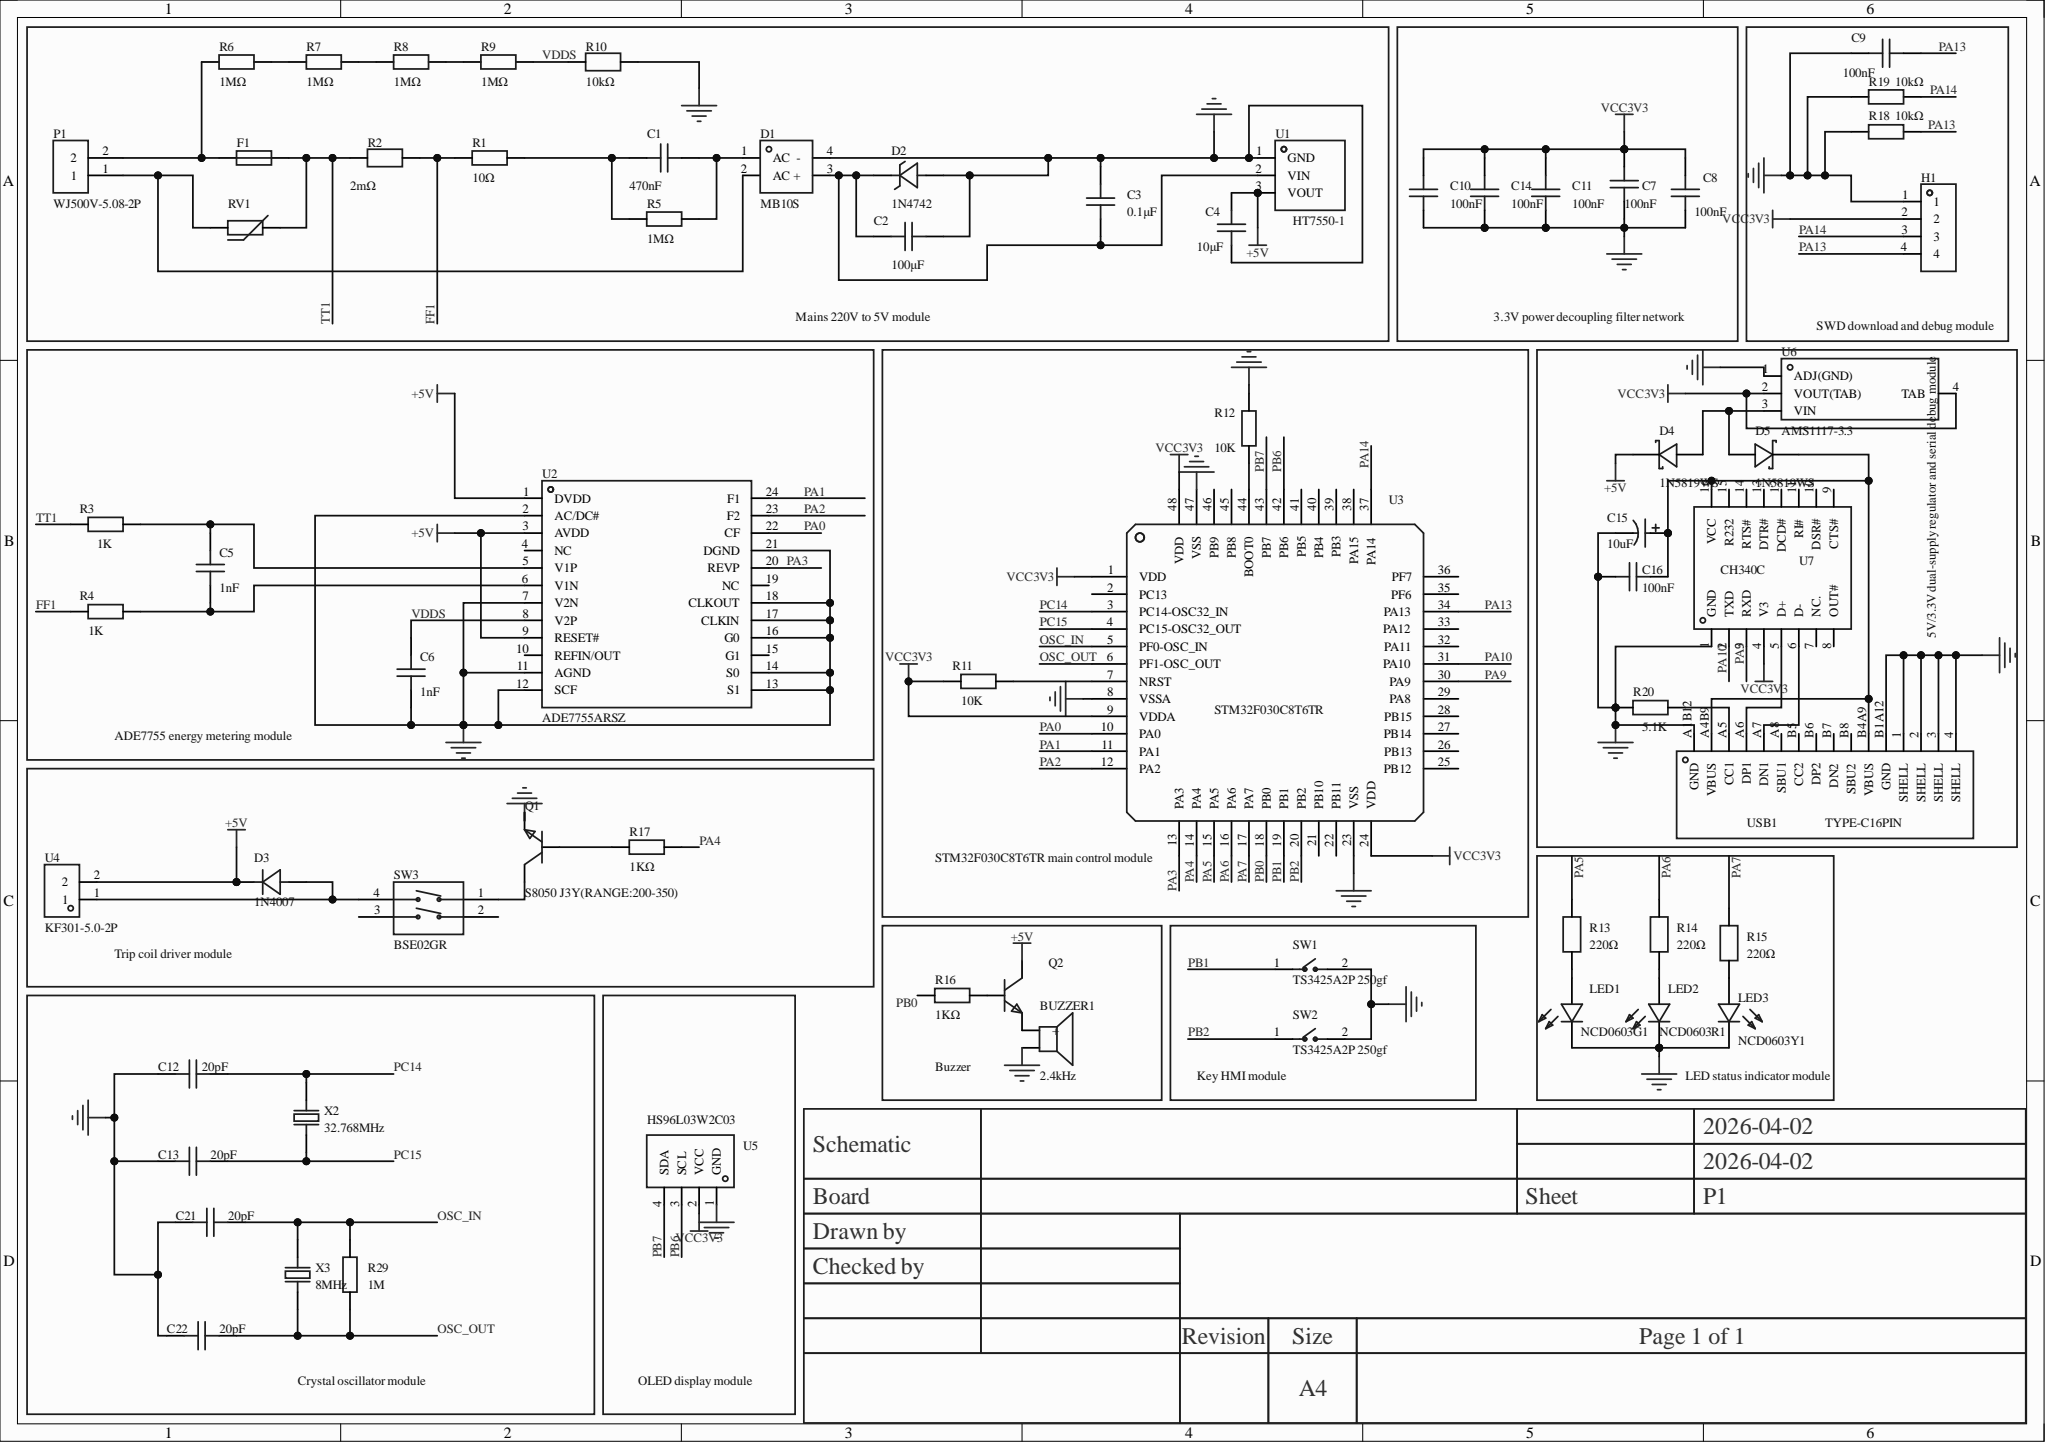Circuit board | Altium Designer | 67 parts | 52 nets
Bill of materials:
Comment,Description,Designator,Footprint,LibRef,Quantity
"2.4kHz","Drive method: active (built-in driver circuit); Construction type: electromagnetic; Rated voltage: 5V; Frequency: 2.4kHz; Sound pressure (SPL): 85dB;","BUZZER1","BUZ-TH_BD12.0-P7.60-D0.6-FD","TMB12A05_C96093","1"
"470nF","Capacitance: 470nF; Tolerance: ±5%; Rated voltage: 400V; Operating temperature: -40℃~+105℃;","C1","CAP-TH_L17.0-W5.5-P15.00-D1.2","CBB21-400V474JP15","1"
"100µF","","C2","C0603","CAP_0603","1"
"0.1µF","","C3","C0603","CAP_0603","1"
"10µF","","C4","C0603","CAP_0603","1"
"1nF","","C5, C6","C0603","CAP_0603","2"
"100nF","Capacitance: 100nF; Tolerance: ±10%; Rated voltage: 50V; Temperature coefficient: X7R;","C7, C8, C10, C14","C0805","GRM21BR71H104KA01L","4"
"100nF","Capacitance: 100nF; Tolerance: ±10%; Rated voltage: 50V; Temperature coefficient: X7R;, [NoValue]","C9, C11, C16","C0603","FCC0603B104K500CT, CAP_0603, CGA0603X7R104K500JT","3"
"20pF","","C12, C13, C21, C22","C0805","CAP_0805","4"
"10uF","Capacitance: 10uF; Tolerance: ±20%; Rated voltage: 50V; Ripple current: 17mA@120Hz; Equivalent series resistance (ESR): -;","C15","CAP-SMD_BD5.0-L5.3-W5.3-FD","RVT1H100M0505_C72487","1"
"MB10S","Forward voltage (Vf): 1.1V@1A; DC reverse withstand voltage (Vr): 1kV; Rectified current: 1A; Non-repetitive peak surge current (Ifsm): 35A;","D1","MBS_L4.7-W4.0-P2.50-LS7.0-TL","MB10S_C42463381","1"
"1N4742","Diode configuration: standalone; Zener voltage (nominal): 12V; Zener voltage (range): 11.45V~12.95V; Power dissipation (Pd): 1W;","D2","DO-41_BD2.4-L4.7-P8.70-D0.8-FD","1N4742","1"
"1N4007","Diode configuration: standalone; Forward voltage (Vf): 1.1V@1A; DC reverse withstand voltage (Vr): 1kV; Rectified current: 1A;","D3","SMA_L4.3-W2.5-LS5.0-RD","1N4007_C727081","1"
"1N5819WS","Forward voltage (Vf): 600mV@1A; DC reverse withstand voltage (Vr): 40V; Rectified current: 1A;","D4, D5","SOD-323_L1.8-W1.3-LS2.5-RD","1N5819WS_C191023","2"
"2F0.05002S1B02","Type: glass tube fuse; Rated current: 500mA; Rated voltage (AC): 250V;125V; Breaking capacity: 50A;","F1","FUSE-TH_BD3.0-L7.2-P11.20-D0.6","2F0.05002S1B02","1"
"","","H1","HDR-TH_4P-P2.54-V-F","HDR-F_2.54_1x4P","1"
"NCD0603G1","Lamp type: -; Light colour: emerald green; Forward voltage (Vf): 2.6V~3.6V; Power: 72mW; Forward current: 20mA; Wavelength: 515nm~530nm; Diode configuration: standalone diode; Lens colour: -; Colour temperature: -; Luminous intensity: 900mcd; Viewing angle: 130°; Packaging: -; Operating temperature: -30℃~+85℃;","LED1","LED0603-RD_1","NCD0603G1","1"
"NCD0603R1","Lamp type: -; Light colour: red; Forward voltage (Vf): 1.6V~2.6V; Power: 65mW; Forward current: 25mA; Wavelength: 615nm~630nm; Diode configuration: standalone diode; Lens colour: -; Colour temperature: -; Luminous intensity: 220mcd; Viewing angle: 130°; Packaging: -; Operating temperature: -30℃~+85℃;","LED2","LED0603-RD_RED","NCD0603R1_C84263","1"
"NCD0603Y1","Lamp type: -; Light colour: yellow; Forward voltage (Vf): 1.6V~2.6V; Power: 65mW; Forward current: 25mA; Wavelength: 586nm~595nm; Diode configuration: standalone diode; Lens colour: -; Colour temperature: -; Luminous intensity: 220mcd; Viewing angle: 130°; Packaging: -; Operating temperature: -30℃~+85℃;","LED3","LED0603-RD","NCD0603Y1","1"
"WJ500V-5.08-2P","Structure: 1x2P; Pitch: 5.08mm; Colour: green; Mounting: through-hole; Rated current: 18A; Rated voltage: 250V; Rows: 1; Wire gauge - AWG: 14~30; Wire gauge - mm²: 2.5; Pins per row: 2; Contact material: -; Contact plating: -; Operating temperature range: -40℃~+105℃; Soldering temperature (max): -;","P1","CONN-TH_2P-P5.00_WJ500V-5.08-2P","WJ500V-5.08-2P","1"
"S8050 J3Y(RANGE:200-350)","Transistor type: NPN; Collector current (Ic): 500mA; Collector-emitter breakdown voltage (Vceo): 25V; Power dissipation (Pd): 300mW; DC current gain (hFE): 200@500mA,1V;","Q1","SOT-23-3_L3.0-W1.7-P0.95-LS2.9-BR","S8050 J3Y(RANGE:200-350)","1"
"","","Q2","S8050_SOT-23","S8050_SOT_NPN","1"
"10Ω","","R1","R0603","Res_0603","1"
"2mΩ","Resistor type: sampling resistor; Resistance: 2mΩ; Tolerance: ±1%; Rated voltage drop: -; Power: 3W; Temperature coefficient: ±50ppm/?; Mounting: SMD;","R2","RES-SMD_L6.4-W3.2-1","HoLLR2512-3W-2mR-1%","1"
"1K","","R3, R4","R0603","Res_0603","2"
"1MΩ","","R5","R0603","Res_0603","1"
"1MΩ","Resistor type: thick film resistor; Resistance: 1MΩ; Tolerance: ±1%; Power: 250mW; Working voltage: 200V; Temperature coefficient: ±100ppm/?;","R6, R7, R8, R9","R1206","1206W4F1004T5E","4"
"10kΩ","Resistor type: metal film resistor; Resistance: 10kΩ; Tolerance: ±1%; Power: 125mW; Working voltage: -; Temperature coefficient: ±50ppm/?;, Resistor type: thick film resistor; Resistance: 10kΩ; Tolerance: ±1%; Power: 125mW; Working voltage: 150V; Temperature coefficient: ±100ppm/?;","R10, R18, R19","R0805","RN73H2ATTD1002F50, 0805W8F1002T5E_C17414","3"
"10K","","R11, R12","R0603","Res_0603","2"
"220Ω","Resistor type: thick film resistor; Resistance: 220Ω; Tolerance: ±1%; Power: 62.5mW; Working voltage: 50V; Temperature coefficient: ±100ppm/?;","R13, R14, R15","R0402","FRC0402F2200TS","3"
"1KΩ","","R16, R17","R0603","Res_0603","2"
"5.1K","","R20","R0603","Res_0603","1"
"1M","","R29","R0805","Res_0805","1"
"190pF@1kHz","Varistor voltage: 423V~517V; Clamping voltage: 775V; Working voltage (DC): 385V; Working voltage (AC): 300V;","RV1","RES-TH_L12.5-W6.7-P7.50-D1.2","10D471K_C8760","1"
"TS3425A2P 250gf","Circuit structure: SPST; Button shape: round button; Actuating force: 2.5N; Mounting: vertical SMD; Switch length: 3.9mm; Switch width: 2.9mm; Switch height: 2.5mm; Bracket: without bracket; Contact current: 50mA; Rated voltage: 12V; Lamp: none; Operating life: 5 ten-thousand cycles;","SW1, SW2","SW-SMD_L3.9-W2.9-LS5.0","TS3425A2P 250gf","2"
"BSE02GR","Circuit structure: SPST; Number of positions: 2; Rated current: 25mA; Rated voltage: 24V; Operating life: 2 thousand cycles; Colour: red;","SW3","SW-TH_4P-L9.9-W6.8-P7.62-BL","BSE02GR","1"
"HT7550-1","Output type: fixed; Operating voltage: 30V; Output voltage: 5V; Output current: 100mA; PSRR: -; Output polarity: positive;","U1","SOT-89_L4.5-W2.5-P1.50-LS4.2-BR","HT7550-1_C347189","1"
"ADE7755ARSZ","Operating voltage: 4.75V~5.25V; Operating current: 3.5mA;","U2","SSOP-24_L8.1-W5.3-P0.65-LS7.8-BL","ADE7755ARSZ","1"
"STM32F030C8T6TR","CPU core: ARM-M0; Max CPU frequency: 48MHz; Application field: -;","U3","LQFP-48_L7.0-W7.0-P0.50-LS9.0-BL","STM32F030C8T6TR","1"
"KF301-5.0-2P","Structure: 1x2P; Pitch: 5mm; Colour: blue; Mounting: through-hole; Rows: 1; Pins per row: 2; Rated current: 17A; Rated voltage: 250V; Wire gauge - AWG: 14~22; Wire gauge - mm²: 1.5; Operating temperature: -30℃~+120℃;","U4","HDR-M-2.54_1X2","KF301-5.0-2P","1"
"HS96L03W2C03","Core chip: SSD1315 chip; Interface type: I2C; Size (inch): 0.96; Pixel resolution: 128x64;","U5","OLED-TH_L27.8-W27.2-P2.54_C9900033791","HS96L03W2C03","1"
"AMS1117-3.3","Output type: fixed; Operating voltage: 12V; Output voltage: 3.3V; Output current: 1A; PSRR: 60dB@(120Hz); Output polarity: positive;","U6","SOT-223-4_L6.5-W3.5-P2.30-LS7.0-BR","AMS1117-3.3_C347222","1"
"CH340C","Application function: transceiver; USB protocol version: USB 2.0; Data rate: 2Mbps;","U7","SOP-16_L10.0-W3.9-P1.27-LS6.0-BL","CH340C","1"
"TYPE-C16PIN","Connector type: Type-C; Protocol standard: -; Gender: female; Mounting: side-mount SMD; Contacts: 16P; Ports: 1; Rated current - power: 3A; Operating temperature: -40℃~+85℃;","USB1","USB-C-SMD_TYPE-C16PIN","TYPE-C16PIN","1"
"32.768MHz","Crystal type: SMD crystal; Frequency: 8MHz; Frequency tolerance at room temperature: ±10ppm; Load capacitance: 12pF; Frequency stability: ±20ppm;","X2","CRYSTAL-SMD_L3.2-W2.5_3225-8MHZ","X22EL89COI-111YLC-8M","1"
"8MHz","Crystal type: SMD crystal; Frequency: 8MHz; Frequency tolerance at room temperature: ±10ppm; Load capacitance: 12pF; Frequency stability: ±20ppm;","X3","CRYSTAL-SMD_L3.2-W2.5_3225-8MHZ","X22EL89COI-111YLC-8M","1"
Netlist (Protel format):
[
BUZZER1
BUZ-TH_BD12.0-P7.60-D0.6-FD
2.4kHz



]
[
C1
CAP-TH_L17.0-W5.5-P15.00-D1.2
470nF



]
[
C2
C0603
100µF



]
[
C3
C0603
0.1µF



]
[
C4
C0603
10µF



]
[
C5
C0603
1nF



]
[
C6
C0603
1nF



]
[
C7
C0805
100nF



]
[
C8
C0805
100nF



]
[
C9
C0603
100nF



]
[
C10
C0805
100nF



]
[
C11
C0603
100nF



]
[
C12
C0805
20pF



]
[
C13
C0805
20pF



]
[
C14
C0805
100nF



]
[
C15
CAP-SMD_BD5.0-L5.3-W5.3-FD
10uF



]
[
C16
C0603
100nF



]
[
C21
C0805
20pF



]
[
C22
C0805
20pF



]
[
D1
MBS_L4.7-W4.0-P2.50-LS7.0-TL
MB10S



]
[
D2
DO-41_BD2.4-L4.7-P8.70-D0.8-FD
1N4742



]
[
D3
SMA_L4.3-W2.5-LS5.0-RD
1N4007



]
[
D4
SOD-323_L1.8-W1.3-LS2.5-RD
1N5819WS



]
[
D5
SOD-323_L1.8-W1.3-LS2.5-RD
1N5819WS



]
[
F1
FUSE-TH_BD3.0-L7.2-P11.20-D0.6
2F.0500212000S1B02



]
[
H1
HDR-TH_4P-P2.54-V-F




]
[
LED1
LED0603-RD_1
NCD0603G1



]
[
LED2
LED0603-RD_RED
NCD0603R1



]
[
LED3
LED0603-RD
NCD0603Y1



]
[
P1
CONN-TH_2P-P5.00_WJ500V-5.08-2P
WJ500V-5.08-2P



]
[
Q1
SOT-23-3_L3.0-W1.7-P0.95-LS2.9-BR
S8050 J3Y(RANGE:200-350)



]
[
Q2
S8050_SOT-23




]
[
R1
R0603
10Ω



]
[
R2
RES-SMD_L6.4-W3.2-1
2mΩ



]
[
R3
R0603
1K



]
[
R4
R0603
1K



]
[
R5
R0603
1MΩ



]
[
R6
R1206
1MΩ



]
[
R7
R1206
1MΩ



]
[
R8
R1206
1MΩ



]
[
R9
R1206
1MΩ



]
[
R10
R0805
10kΩ



]
[
R11
R0603
10K



]
[
R12
R0603
10K



]
[
R13
R0402
220Ω



]
[
R14
R0402
220Ω



]
[
R15
R0402
220Ω



]
[
R16
R0603
1KΩ



]
[
R17
R0603
1KΩ



]
[
R18
R0805
10kΩ



]
[
R19
R0805
10kΩ



]
[
R20
R0603
5.1K



]
[
R29
R0805
1M



]
[
RV1
RES-TH_L12.5-W6.7-P7.50-D1.2
190pF@1kHz



]
[
SW1
SW-SMD_L3.9-W2.9-LS5.0
TS3425A2P 250gf



]
[
SW2
SW-SMD_L3.9-W2.9-LS5.0
TS3425A2P 250gf



]
[
SW3
SW-TH_4P-L9.9-W6.8-P7.62-BL
BSE02GR



]
[
U1
SOT-89_L4.5-W2.5-P1.50-LS4.2-BR
HT7550-1



]
[
U2
SSOP-24_L8.1-W5.3-P0.65-LS7.8-BL
ADE7755ARSZ



]
[
U3
LQFP-48_L7.0-W7.0-P0.50-LS9.0-BL
STM32F030C8T6TR



]
[
U4
HDR-M-2.54_1X2
KF301-5.0-2P



]
[
U5
OLED-TH_L27.8-W27.2-P2.54_C9900033791
HS96L03W2C03



]
[
U6
SOT-223-4_L6.5-W3.5-P2.30-LS7.0-BR
AMS1117-3.3



]
[
U7
SOP-16_L10.0-W3.9-P1.27-LS6.0-BL
CH340C



]
[
USB1
USB-C-SMD_TYPE-C16PIN
TYPE-C16PIN



]
[
X2
CRYSTAL-SMD_L3.2-W2.5_3225-8MHZ
32.768MHz



]
[
X3
CRYSTAL-SMD_L3.2-W2.5_3225-8MHZ
8MHz



]
(
VDDS
C6-2
R9-2
R10-1
U2-8
)
(
VCC3V3
C7-1
C8-2
C10-1
C11-2
C14-2
H1-2
R11-1
U3-1
U3-9
U3-24
U3-48
U5-2
U6-2
U6-4
U7-4
)
(
TT1
F1-2
R2-1
R3-1
RV1-2
)
(
PC15
C13-2
U3-4
X2-1
)
(
PC14
C12-1
U3-3
X2-2
)
(
PB7
U3-43
U5-4
)
(
PB6
U3-42
U5-3
)
(
PB2
SW2-1
U3-20
)
(
PB1
SW1-1
U3-19
)
(
PB0
R16-2
U3-18
)
(
PA14
H1-3
R19-1
U3-37
)
(
PA13
C9-2
H1-4
R18-1
U3-34
)
(
PA10
U3-31
U7-2
)
(
PA9
U3-30
U7-3
)
(
PA7
R15-2
U3-17
)
(
PA6
R14-2
U3-16
)
(
PA5
R13-2
U3-15
)
(
PA4
R17-1
U3-14
)
(
PA3
U2-20
U3-13
)
(
PA2
U2-23
U3-12
)
(
PA1
U2-24
U3-11
)
(
PA0
U2-22
U3-10
)
(
OSC_OUT
C22-2
R29-1
U3-6
X3-1
)
(
OSC_IN
C21-2
R29-2
U3-5
X3-2
)
(
NetU7_6
U7-6
USB1-A7
)
(
NetU7_5
U7-5
USB1-A6
)
(
NetR20_1
R20-1
USB1-A5
)
(
NetR12_1
R12-1
U3-44
)
(
NetR11_2
R11-2
U3-7
)
(
NetR8_2
R8-2
R9-1
)
(
NetR7_2
R7-2
R8-1
)
(
NetR6_2
R6-2
R7-1
)
(
NetQ2_1
Q2-1
R16-1
)
(
NetQ1_3
Q1-3
SW3-1
)
(
NetQ1_1
Q1-1
R17-2
)
(
NetLED3_2
LED3-2
R15-1
)
(
NetLED2_2
LED2-2
R14-1
)
(
NetLED1_2
LED1-2
R13-1
)
(
NetF1_1
F1-1
P1-2
R6-1
)
(
NetD4_2
D4-2
D5-2
U6-3
)
(
NetD3_2
D3-2
SW3-4
U4-1
)
(
NetD1_2
D1-2
P1-1
RV1-1
)
(
NetC15_1
C15-1
C16-2
D5-1
U7-16
USB1-A4B9
USB1-B4A9
)
(
NetC5_2
C5-2
R3-2
U2-5
)
(
NetC5_1
C5-1
R4-2
U2-6
)
(
NetC2_2
C2-2
C3-1
D1-3
D2-2
U1-2
)
(
NetC1_2
C1-2
R1-2
R5-1
)
(
NetC1_1
C1-1
D1-1
R5-2
)
(
NetBUZZER1_1
BUZZER1-1
Q2-2
)
(
GND
BUZZER1-2
C2-1
C3-2
C4-1
C6-1
C7-2
C8-1
C9-1
C10-2
C11-1
C12-2
C13-1
C14-1
C15-2
C16-1
C21-1
C22-1
D1-4
D2-1
H1-1
LED1-1
LED2-1
LED3-1
Q1-2
R10-2
R12-2
R18-2
R19-2
R20-2
SW1-2
SW2-2
U1-1
U2-2
U2-7
U2-11
U2-12
U2-13
U2-14
U2-16
U2-17
U2-18
U2-21
U3-8
U3-23
U3-47
U5-1
U6-1
U7-1
USB1-1
USB1-2
USB1-3
USB1-4
USB1-A1B12
USB1-B1A12
)
(
FF1
R1-1
R2-2
R4-1
)
(
+5V
C4-2
D3-1
D4-1
Q2-3
U1-3
U2-1
U2-3
U2-9
U4-2
)